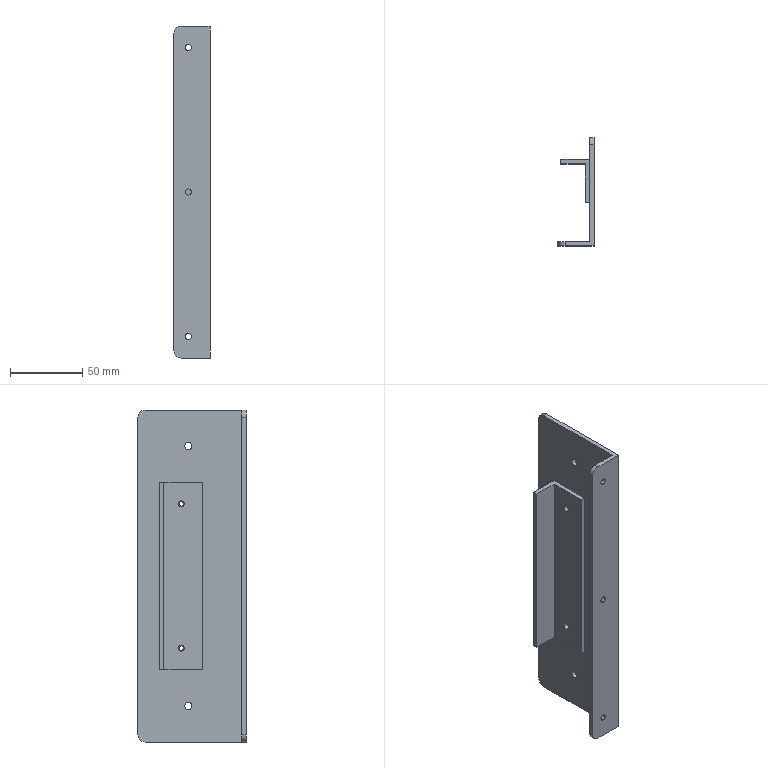Part | SolidWorks | features HoleWzd 4, Fillet 2, FlattenBends 2, ProcessBends 2, BossThin 1, ExtruThin 1 | 2 solids | 38 faces | box 25 x 75 x 230 mm | volume 84822 mm3 | cylinder 22 | plane 16 | commonest cylinder face diameters 4.2 x10 3.2 x4 5 x4 10 x4
STEP:
#1=CARTESIAN_POINT('',(22.,45.,-47.9));
#2=VERTEX_POINT('',#1);
#3=CARTESIAN_POINT('',(22.,45.,-52.1));
#4=VERTEX_POINT('',#3);
#5=CARTESIAN_POINT('',(22.,45.,-50.));
#6=DIRECTION('',(1.,0.,0.));
#7=DIRECTION('',(0.,1.,0.));
#8=AXIS2_PLACEMENT_3D('',#5,#6,#7);
#9=CIRCLE('',#8,2.1);
#10=EDGE_CURVE('',#2,#4,#9,.T.);
#11=ORIENTED_EDGE('',*,*,#10,.T.);
#12=CARTESIAN_POINT('',(19.,45.,-52.1));
#13=VERTEX_POINT('',#12);
#14=CARTESIAN_POINT('',(19.,45.,-52.1));
#15=DIRECTION('',(-1.,0.,0.));
#16=VECTOR('',#15,1000.);
#17=LINE('',#14,#16);
#18=EDGE_CURVE('',#4,#13,#17,.T.);
#19=ORIENTED_EDGE('',*,*,#18,.T.);
#20=CARTESIAN_POINT('',(19.,45.,-47.9));
#21=VERTEX_POINT('',#20);
#22=CARTESIAN_POINT('',(19.,45.,-50.));
#23=DIRECTION('',(-1.,0.,0.));
#24=DIRECTION('',(0.,0.,1.));
#25=AXIS2_PLACEMENT_3D('',#22,#23,#24);
#26=CIRCLE('',#25,2.1);
#27=EDGE_CURVE('',#13,#21,#26,.T.);
#28=ORIENTED_EDGE('',*,*,#27,.T.);
#29=CARTESIAN_POINT('',(19.,45.,-47.9));
#30=DIRECTION('',(-1.,0.,0.));
#31=VECTOR('',#30,1000.);
#32=LINE('',#29,#31);
#33=EDGE_CURVE('',#2,#21,#32,.T.);
#34=ORIENTED_EDGE('',*,*,#33,.F.);
#35=EDGE_LOOP('',(#11,#19,#28,#34));
#36=FACE_OUTER_BOUND('',#35,.T.);
#37=CARTESIAN_POINT('',(19.,45.,-50.));
#38=DIRECTION('',(-1.,0.,0.));
#39=DIRECTION('',(0.,0.,1.));
#40=AXIS2_PLACEMENT_3D('',#37,#38,#39);
#41=CYLINDRICAL_SURFACE('',#40,2.1);
#42=ADVANCED_FACE('',(#36),#41,.F.);
#43=CARTESIAN_POINT('',(22.,45.,52.1));
#44=VERTEX_POINT('',#43);
#45=CARTESIAN_POINT('',(22.,45.,47.9));
#46=VERTEX_POINT('',#45);
#47=CARTESIAN_POINT('',(22.,45.,50.));
#48=DIRECTION('',(1.,0.,0.));
#49=DIRECTION('',(0.,1.,0.));
#50=AXIS2_PLACEMENT_3D('',#47,#48,#49);
#51=CIRCLE('',#50,2.1);
#52=EDGE_CURVE('',#44,#46,#51,.T.);
#53=ORIENTED_EDGE('',*,*,#52,.T.);
#54=CARTESIAN_POINT('',(19.,45.,47.9));
#55=VERTEX_POINT('',#54);
#56=CARTESIAN_POINT('',(19.,45.,47.9));
#57=DIRECTION('',(-1.,0.,0.));
#58=VECTOR('',#57,1000.);
#59=LINE('',#56,#58);
#60=EDGE_CURVE('',#46,#55,#59,.T.);
#61=ORIENTED_EDGE('',*,*,#60,.T.);
#62=CARTESIAN_POINT('',(19.,45.,52.1));
#63=VERTEX_POINT('',#62);
#64=CARTESIAN_POINT('',(19.,45.,50.));
#65=DIRECTION('',(-1.,0.,0.));
#66=DIRECTION('',(0.,0.,1.));
#67=AXIS2_PLACEMENT_3D('',#64,#65,#66);
#68=CIRCLE('',#67,2.1);
#69=EDGE_CURVE('',#55,#63,#68,.T.);
#70=ORIENTED_EDGE('',*,*,#69,.T.);
#71=CARTESIAN_POINT('',(19.,45.,52.1));
#72=DIRECTION('',(-1.,0.,0.));
#73=VECTOR('',#72,1000.);
#74=LINE('',#71,#73);
#75=EDGE_CURVE('',#44,#63,#74,.T.);
#76=ORIENTED_EDGE('',*,*,#75,.F.);
#77=EDGE_LOOP('',(#53,#61,#70,#76));
#78=FACE_OUTER_BOUND('',#77,.T.);
#79=CARTESIAN_POINT('',(19.,45.,50.));
#80=DIRECTION('',(-1.,0.,0.));
#81=DIRECTION('',(0.,0.,1.));
#82=AXIS2_PLACEMENT_3D('',#79,#80,#81);
#83=CYLINDRICAL_SURFACE('',#82,2.1);
#84=ADVANCED_FACE('',(#78),#83,.F.);
#85=CARTESIAN_POINT('',(19.,45.,-50.));
#86=DIRECTION('',(-1.,0.,0.));
#87=DIRECTION('',(0.,0.,1.));
#88=AXIS2_PLACEMENT_3D('',#85,#86,#87);
#89=CIRCLE('',#88,2.1);
#90=EDGE_CURVE('',#21,#13,#89,.T.);
#91=ORIENTED_EDGE('',*,*,#90,.F.);
#92=ORIENTED_EDGE('',*,*,#27,.F.);
#93=EDGE_LOOP('',(#91,#92));
#94=FACE_BOUND('',#93,.T.);
#95=CARTESIAN_POINT('',(19.,45.,50.));
#96=DIRECTION('',(-1.,0.,0.));
#97=DIRECTION('',(0.,0.,1.));
#98=AXIS2_PLACEMENT_3D('',#95,#96,#97);
#99=CIRCLE('',#98,2.1);
#100=EDGE_CURVE('',#63,#55,#99,.T.);
#101=ORIENTED_EDGE('',*,*,#100,.F.);
#102=ORIENTED_EDGE('',*,*,#69,.F.);
#103=EDGE_LOOP('',(#101,#102));
#104=FACE_BOUND('',#103,.T.);
#105=CARTESIAN_POINT('',(19.,57.,-65.));
#106=VERTEX_POINT('',#105);
#107=CARTESIAN_POINT('',(19.,30.,-65.));
#108=VERTEX_POINT('',#107);
#109=CARTESIAN_POINT('',(19.,60.,-65.));
#110=DIRECTION('',(0.,-1.,0.));
#111=VECTOR('',#110,1000.);
#112=LINE('',#109,#111);
#113=EDGE_CURVE('',#106,#108,#112,.T.);
#114=ORIENTED_EDGE('',*,*,#113,.T.);
#115=CARTESIAN_POINT('',(19.,30.,65.));
#116=VERTEX_POINT('',#115);
#117=CARTESIAN_POINT('',(19.,30.,65.));
#118=DIRECTION('',(0.,0.,-1.));
#119=VECTOR('',#118,1000.);
#120=LINE('',#117,#119);
#121=EDGE_CURVE('',#116,#108,#120,.T.);
#122=ORIENTED_EDGE('',*,*,#121,.F.);
#123=CARTESIAN_POINT('',(19.,57.,65.));
#124=VERTEX_POINT('',#123);
#125=CARTESIAN_POINT('',(19.,60.,65.));
#126=DIRECTION('',(0.,-1.,0.));
#127=VECTOR('',#126,1000.);
#128=LINE('',#125,#127);
#129=EDGE_CURVE('',#124,#116,#128,.T.);
#130=ORIENTED_EDGE('',*,*,#129,.F.);
#131=CARTESIAN_POINT('',(19.,57.,65.));
#132=DIRECTION('',(0.,0.,-1.));
#133=VECTOR('',#132,1000.);
#134=LINE('',#131,#133);
#135=EDGE_CURVE('',#124,#106,#134,.T.);
#136=ORIENTED_EDGE('',*,*,#135,.T.);
#137=EDGE_LOOP('',(#114,#122,#130,#136));
#138=FACE_OUTER_BOUND('',#137,.T.);
#139=CARTESIAN_POINT('',(19.,60.,65.));
#140=DIRECTION('',(1.,0.,0.));
#141=DIRECTION('',(0.,1.,0.));
#142=AXIS2_PLACEMENT_3D('',#139,#140,#141);
#143=PLANE('',#142);
#144=ADVANCED_FACE('',(#94,#104,#138),#143,.F.);
#145=CARTESIAN_POINT('',(22.,30.,-65.));
#146=VERTEX_POINT('',#145);
#147=CARTESIAN_POINT('',(22.,30.,-65.));
#148=DIRECTION('',(-1.,0.,0.));
#149=VECTOR('',#148,1000.);
#150=LINE('',#147,#149);
#151=EDGE_CURVE('',#146,#108,#150,.T.);
#152=ORIENTED_EDGE('',*,*,#151,.F.);
#153=CARTESIAN_POINT('',(22.,30.,65.));
#154=VERTEX_POINT('',#153);
#155=CARTESIAN_POINT('',(22.,30.,65.));
#156=DIRECTION('',(0.,0.,-1.));
#157=VECTOR('',#156,1000.);
#158=LINE('',#155,#157);
#159=EDGE_CURVE('',#154,#146,#158,.T.);
#160=ORIENTED_EDGE('',*,*,#159,.F.);
#161=CARTESIAN_POINT('',(22.,30.,65.));
#162=DIRECTION('',(-1.,0.,0.));
#163=VECTOR('',#162,1000.);
#164=LINE('',#161,#163);
#165=EDGE_CURVE('',#154,#116,#164,.T.);
#166=ORIENTED_EDGE('',*,*,#165,.T.);
#167=ORIENTED_EDGE('',*,*,#121,.T.);
#168=EDGE_LOOP('',(#152,#160,#166,#167));
#169=FACE_OUTER_BOUND('',#168,.T.);
#170=CARTESIAN_POINT('',(22.,30.,65.));
#171=DIRECTION('',(0.,-1.,0.));
#172=DIRECTION('',(0.,0.,-1.));
#173=AXIS2_PLACEMENT_3D('',#170,#171,#172);
#174=PLANE('',#173);
#175=ADVANCED_FACE('',(#169),#174,.T.);
#176=ORIENTED_EDGE('',*,*,#10,.F.);
#177=CARTESIAN_POINT('',(22.,45.,-50.));
#178=DIRECTION('',(1.,0.,0.));
#179=DIRECTION('',(0.,1.,0.));
#180=AXIS2_PLACEMENT_3D('',#177,#178,#179);
#181=CIRCLE('',#180,2.1);
#182=EDGE_CURVE('',#4,#2,#181,.T.);
#183=ORIENTED_EDGE('',*,*,#182,.F.);
#184=EDGE_LOOP('',(#176,#183));
#185=FACE_BOUND('',#184,.T.);
#186=ORIENTED_EDGE('',*,*,#52,.F.);
#187=CARTESIAN_POINT('',(22.,45.,50.));
#188=DIRECTION('',(1.,0.,0.));
#189=DIRECTION('',(0.,1.,0.));
#190=AXIS2_PLACEMENT_3D('',#187,#188,#189);
#191=CIRCLE('',#190,2.1);
#192=EDGE_CURVE('',#46,#44,#191,.T.);
#193=ORIENTED_EDGE('',*,*,#192,.F.);
#194=EDGE_LOOP('',(#186,#193));
#195=FACE_BOUND('',#194,.T.);
#196=CARTESIAN_POINT('',(22.,60.,-65.));
#197=VERTEX_POINT('',#196);
#198=CARTESIAN_POINT('',(22.,60.,-65.));
#199=DIRECTION('',(0.,-1.,0.));
#200=VECTOR('',#199,1000.);
#201=LINE('',#198,#200);
#202=EDGE_CURVE('',#197,#146,#201,.T.);
#203=ORIENTED_EDGE('',*,*,#202,.F.);
#204=CARTESIAN_POINT('',(22.,60.,65.));
#205=VERTEX_POINT('',#204);
#206=CARTESIAN_POINT('',(22.,60.,65.));
#207=DIRECTION('',(0.,0.,-1.));
#208=VECTOR('',#207,1000.);
#209=LINE('',#206,#208);
#210=EDGE_CURVE('',#205,#197,#209,.T.);
#211=ORIENTED_EDGE('',*,*,#210,.F.);
#212=CARTESIAN_POINT('',(22.,60.,65.));
#213=DIRECTION('',(0.,-1.,0.));
#214=VECTOR('',#213,1000.);
#215=LINE('',#212,#214);
#216=EDGE_CURVE('',#205,#154,#215,.T.);
#217=ORIENTED_EDGE('',*,*,#216,.T.);
#218=ORIENTED_EDGE('',*,*,#159,.T.);
#219=EDGE_LOOP('',(#203,#211,#217,#218));
#220=FACE_OUTER_BOUND('',#219,.T.);
#221=CARTESIAN_POINT('',(22.,60.,65.));
#222=DIRECTION('',(1.,0.,0.));
#223=DIRECTION('',(0.,1.,0.));
#224=AXIS2_PLACEMENT_3D('',#221,#222,#223);
#225=PLANE('',#224);
#226=ADVANCED_FACE('',(#185,#195,#220),#225,.T.);
#227=CARTESIAN_POINT('',(2.,60.,-65.));
#228=VERTEX_POINT('',#227);
#229=CARTESIAN_POINT('',(2.,60.,-65.));
#230=DIRECTION('',(1.,0.,0.));
#231=VECTOR('',#230,1000.);
#232=LINE('',#229,#231);
#233=EDGE_CURVE('',#228,#197,#232,.T.);
#234=ORIENTED_EDGE('',*,*,#233,.F.);
#235=CARTESIAN_POINT('',(2.,60.,65.));
#236=VERTEX_POINT('',#235);
#237=CARTESIAN_POINT('',(2.,60.,65.));
#238=DIRECTION('',(0.,0.,-1.));
#239=VECTOR('',#238,1000.);
#240=LINE('',#237,#239);
#241=EDGE_CURVE('',#236,#228,#240,.T.);
#242=ORIENTED_EDGE('',*,*,#241,.F.);
#243=CARTESIAN_POINT('',(2.,60.,65.));
#244=DIRECTION('',(1.,0.,0.));
#245=VECTOR('',#244,1000.);
#246=LINE('',#243,#245);
#247=EDGE_CURVE('',#236,#205,#246,.T.);
#248=ORIENTED_EDGE('',*,*,#247,.T.);
#249=ORIENTED_EDGE('',*,*,#210,.T.);
#250=EDGE_LOOP('',(#234,#242,#248,#249));
#251=FACE_OUTER_BOUND('',#250,.T.);
#252=CARTESIAN_POINT('',(2.,60.,65.));
#253=DIRECTION('',(0.,1.,0.));
#254=DIRECTION('',(0.,0.,1.));
#255=AXIS2_PLACEMENT_3D('',#252,#253,#254);
#256=PLANE('',#255);
#257=ADVANCED_FACE('',(#251),#256,.T.);
#258=CARTESIAN_POINT('',(2.,57.,-65.));
#259=VERTEX_POINT('',#258);
#260=CARTESIAN_POINT('',(2.,57.,-65.));
#261=DIRECTION('',(0.,1.,0.));
#262=VECTOR('',#261,1000.);
#263=LINE('',#260,#262);
#264=EDGE_CURVE('',#259,#228,#263,.T.);
#265=ORIENTED_EDGE('',*,*,#264,.F.);
#266=CARTESIAN_POINT('',(2.,57.,65.));
#267=VERTEX_POINT('',#266);
#268=CARTESIAN_POINT('',(2.,57.,65.));
#269=DIRECTION('',(0.,0.,-1.));
#270=VECTOR('',#269,1000.);
#271=LINE('',#268,#270);
#272=EDGE_CURVE('',#267,#259,#271,.T.);
#273=ORIENTED_EDGE('',*,*,#272,.F.);
#274=CARTESIAN_POINT('',(2.,57.,65.));
#275=DIRECTION('',(0.,1.,0.));
#276=VECTOR('',#275,1000.);
#277=LINE('',#274,#276);
#278=EDGE_CURVE('',#267,#236,#277,.T.);
#279=ORIENTED_EDGE('',*,*,#278,.T.);
#280=ORIENTED_EDGE('',*,*,#241,.T.);
#281=EDGE_LOOP('',(#265,#273,#279,#280));
#282=FACE_OUTER_BOUND('',#281,.T.);
#283=CARTESIAN_POINT('',(2.,57.,65.));
#284=DIRECTION('',(-1.,0.,0.));
#285=DIRECTION('',(0.,0.,1.));
#286=AXIS2_PLACEMENT_3D('',#283,#284,#285);
#287=PLANE('',#286);
#288=ADVANCED_FACE('',(#282),#287,.T.);
#289=CARTESIAN_POINT('',(2.,57.,-65.));
#290=DIRECTION('',(1.,0.,0.));
#291=VECTOR('',#290,1000.);
#292=LINE('',#289,#291);
#293=EDGE_CURVE('',#259,#106,#292,.T.);
#294=ORIENTED_EDGE('',*,*,#293,.T.);
#295=ORIENTED_EDGE('',*,*,#135,.F.);
#296=CARTESIAN_POINT('',(2.,57.,65.));
#297=DIRECTION('',(1.,0.,0.));
#298=VECTOR('',#297,1000.);
#299=LINE('',#296,#298);
#300=EDGE_CURVE('',#267,#124,#299,.T.);
#301=ORIENTED_EDGE('',*,*,#300,.F.);
#302=ORIENTED_EDGE('',*,*,#272,.T.);
#303=EDGE_LOOP('',(#294,#295,#301,#302));
#304=FACE_OUTER_BOUND('',#303,.T.);
#305=CARTESIAN_POINT('',(2.,57.,65.));
#306=DIRECTION('',(0.,1.,0.));
#307=DIRECTION('',(0.,0.,1.));
#308=AXIS2_PLACEMENT_3D('',#305,#306,#307);
#309=PLANE('',#308);
#310=ADVANCED_FACE('',(#304),#309,.F.);
#311=ORIENTED_EDGE('',*,*,#129,.T.);
#312=ORIENTED_EDGE('',*,*,#165,.F.);
#313=ORIENTED_EDGE('',*,*,#216,.F.);
#314=ORIENTED_EDGE('',*,*,#247,.F.);
#315=ORIENTED_EDGE('',*,*,#278,.F.);
#316=ORIENTED_EDGE('',*,*,#300,.T.);
#317=EDGE_LOOP('',(#311,#312,#313,#314,#315,#316));
#318=FACE_OUTER_BOUND('',#317,.T.);
#319=CARTESIAN_POINT('',(0.,0.,65.));
#320=DIRECTION('',(0.,0.,-1.));
#321=DIRECTION('',(-1.,0.,0.));
#322=AXIS2_PLACEMENT_3D('',#319,#320,#321);
#323=PLANE('',#322);
#324=ADVANCED_FACE('',(#318),#323,.F.);
#325=ORIENTED_EDGE('',*,*,#113,.F.);
#326=ORIENTED_EDGE('',*,*,#293,.F.);
#327=ORIENTED_EDGE('',*,*,#264,.T.);
#328=ORIENTED_EDGE('',*,*,#233,.T.);
#329=ORIENTED_EDGE('',*,*,#202,.T.);
#330=ORIENTED_EDGE('',*,*,#151,.T.);
#331=EDGE_LOOP('',(#325,#326,#327,#328,#329,#330));
#332=FACE_OUTER_BOUND('',#331,.T.);
#333=CARTESIAN_POINT('',(0.,0.,-65.));
#334=DIRECTION('',(0.,0.,-1.));
#335=DIRECTION('',(-1.,0.,0.));
#336=AXIS2_PLACEMENT_3D('',#333,#334,#335);
#337=PLANE('',#336);
#338=ADVANCED_FACE('',(#332),#337,.T.);
#339=ORIENTED_EDGE('',*,*,#60,.F.);
#340=ORIENTED_EDGE('',*,*,#192,.T.);
#341=ORIENTED_EDGE('',*,*,#75,.T.);
#342=ORIENTED_EDGE('',*,*,#100,.T.);
#343=EDGE_LOOP('',(#339,#340,#341,#342));
#344=FACE_OUTER_BOUND('',#343,.T.);
#345=CARTESIAN_POINT('',(19.,45.,50.));
#346=DIRECTION('',(-1.,0.,0.));
#347=DIRECTION('',(0.,0.,1.));
#348=AXIS2_PLACEMENT_3D('',#345,#346,#347);
#349=CYLINDRICAL_SURFACE('',#348,2.1);
#350=ADVANCED_FACE('',(#344),#349,.F.);
#351=ORIENTED_EDGE('',*,*,#18,.F.);
#352=ORIENTED_EDGE('',*,*,#182,.T.);
#353=ORIENTED_EDGE('',*,*,#33,.T.);
#354=ORIENTED_EDGE('',*,*,#90,.T.);
#355=EDGE_LOOP('',(#351,#352,#353,#354));
#356=FACE_OUTER_BOUND('',#355,.T.);
#357=CARTESIAN_POINT('',(19.,45.,-50.));
#358=DIRECTION('',(-1.,0.,0.));
#359=DIRECTION('',(0.,0.,1.));
#360=AXIS2_PLACEMENT_3D('',#357,#358,#359);
#361=CYLINDRICAL_SURFACE('',#360,2.1);
#362=ADVANCED_FACE('',(#356),#361,.F.);
#363=CLOSED_SHELL('',(#42,#84,#144,#175,#226,#257,#288,#310,#324,#338,#350,#362));
#364=MANIFOLD_SOLID_BREP('',#363);
#365=CARTESIAN_POINT('',(25.,45.,-51.6));
#366=VERTEX_POINT('',#365);
#367=CARTESIAN_POINT('',(25.,45.,-48.4));
#368=VERTEX_POINT('',#367);
#369=CARTESIAN_POINT('',(25.,45.,-50.));
#370=DIRECTION('',(-1.,0.,0.));
#371=DIRECTION('',(0.,0.,1.));
#372=AXIS2_PLACEMENT_3D('',#369,#370,#371);
#373=CIRCLE('',#372,1.6);
#374=EDGE_CURVE('',#366,#368,#373,.T.);
#375=ORIENTED_EDGE('',*,*,#374,.F.);
#376=CARTESIAN_POINT('',(22.,45.,-51.6));
#377=VERTEX_POINT('',#376);
#378=CARTESIAN_POINT('',(22.,45.,-51.6));
#379=DIRECTION('',(-1.,0.,0.));
#380=VECTOR('',#379,1000.);
#381=LINE('',#378,#380);
#382=EDGE_CURVE('',#366,#377,#381,.T.);
#383=ORIENTED_EDGE('',*,*,#382,.T.);
#384=CARTESIAN_POINT('',(22.,45.,-48.4));
#385=VERTEX_POINT('',#384);
#386=CARTESIAN_POINT('',(22.,45.,-50.));
#387=DIRECTION('',(-1.,0.,0.));
#388=DIRECTION('',(0.,0.,1.));
#389=AXIS2_PLACEMENT_3D('',#386,#387,#388);
#390=CIRCLE('',#389,1.6);
#391=EDGE_CURVE('',#377,#385,#390,.T.);
#392=ORIENTED_EDGE('',*,*,#391,.T.);
#393=CARTESIAN_POINT('',(22.,45.,-48.4));
#394=DIRECTION('',(-1.,0.,0.));
#395=VECTOR('',#394,1000.);
#396=LINE('',#393,#395);
#397=EDGE_CURVE('',#368,#385,#396,.T.);
#398=ORIENTED_EDGE('',*,*,#397,.F.);
#399=EDGE_LOOP('',(#375,#383,#392,#398));
#400=FACE_OUTER_BOUND('',#399,.T.);
#401=CARTESIAN_POINT('',(22.,45.,-50.));
#402=DIRECTION('',(-1.,0.,0.));
#403=DIRECTION('',(0.,0.,1.));
#404=AXIS2_PLACEMENT_3D('',#401,#402,#403);
#405=CYLINDRICAL_SURFACE('',#404,1.6);
#406=ADVANCED_FACE('',(#400),#405,.F.);
#407=CARTESIAN_POINT('',(25.,45.,48.4));
#408=VERTEX_POINT('',#407);
#409=CARTESIAN_POINT('',(25.,45.,51.6));
#410=VERTEX_POINT('',#409);
#411=CARTESIAN_POINT('',(25.,45.,50.));
#412=DIRECTION('',(-1.,0.,0.));
#413=DIRECTION('',(0.,0.,1.));
#414=AXIS2_PLACEMENT_3D('',#411,#412,#413);
#415=CIRCLE('',#414,1.6);
#416=EDGE_CURVE('',#408,#410,#415,.T.);
#417=ORIENTED_EDGE('',*,*,#416,.F.);
#418=CARTESIAN_POINT('',(22.,45.,48.4));
#419=VERTEX_POINT('',#418);
#420=CARTESIAN_POINT('',(22.,45.,48.4));
#421=DIRECTION('',(-1.,0.,0.));
#422=VECTOR('',#421,1000.);
#423=LINE('',#420,#422);
#424=EDGE_CURVE('',#408,#419,#423,.T.);
#425=ORIENTED_EDGE('',*,*,#424,.T.);
#426=CARTESIAN_POINT('',(22.,45.,51.6));
#427=VERTEX_POINT('',#426);
#428=CARTESIAN_POINT('',(22.,45.,50.));
#429=DIRECTION('',(-1.,0.,0.));
#430=DIRECTION('',(0.,0.,1.));
#431=AXIS2_PLACEMENT_3D('',#428,#429,#430);
#432=CIRCLE('',#431,1.6);
#433=EDGE_CURVE('',#419,#427,#432,.T.);
#434=ORIENTED_EDGE('',*,*,#433,.T.);
#435=CARTESIAN_POINT('',(22.,45.,51.6));
#436=DIRECTION('',(-1.,0.,0.));
#437=VECTOR('',#436,1000.);
#438=LINE('',#435,#437);
#439=EDGE_CURVE('',#410,#427,#438,.T.);
#440=ORIENTED_EDGE('',*,*,#439,.F.);
#441=EDGE_LOOP('',(#417,#425,#434,#440));
#442=FACE_OUTER_BOUND('',#441,.T.);
#443=CARTESIAN_POINT('',(22.,45.,50.));
#444=DIRECTION('',(-1.,0.,0.));
#445=DIRECTION('',(0.,0.,1.));
#446=AXIS2_PLACEMENT_3D('',#443,#444,#445);
#447=CYLINDRICAL_SURFACE('',#446,1.6);
#448=ADVANCED_FACE('',(#442),#447,.F.);
#449=CARTESIAN_POINT('',(25.,40.,-92.5));
#450=VERTEX_POINT('',#449);
#451=CARTESIAN_POINT('',(25.,40.,-87.5));
#452=VERTEX_POINT('',#451);
#453=CARTESIAN_POINT('',(25.,40.,-90.));
#454=DIRECTION('',(-1.,0.,0.));
#455=DIRECTION('',(0.,0.,1.));
#456=AXIS2_PLACEMENT_3D('',#453,#454,#455);
#457=CIRCLE('',#456,2.5);
#458=EDGE_CURVE('',#450,#452,#457,.T.);
#459=ORIENTED_EDGE('',*,*,#458,.F.);
#460=CARTESIAN_POINT('',(22.,40.,-92.5));
#461=VERTEX_POINT('',#460);
#462=CARTESIAN_POINT('',(22.,40.,-92.5));
#463=DIRECTION('',(-1.,0.,0.));
#464=VECTOR('',#463,1000.);
#465=LINE('',#462,#464);
#466=EDGE_CURVE('',#450,#461,#465,.T.);
#467=ORIENTED_EDGE('',*,*,#466,.T.);
#468=CARTESIAN_POINT('',(22.,40.,-87.5));
#469=VERTEX_POINT('',#468);
#470=CARTESIAN_POINT('',(22.,40.,-90.));
#471=DIRECTION('',(-1.,0.,0.));
#472=DIRECTION('',(0.,0.,1.));
#473=AXIS2_PLACEMENT_3D('',#470,#471,#472);
#474=CIRCLE('',#473,2.5);
#475=EDGE_CURVE('',#461,#469,#474,.T.);
#476=ORIENTED_EDGE('',*,*,#475,.T.);
#477=CARTESIAN_POINT('',(22.,40.,-87.5));
#478=DIRECTION('',(-1.,0.,0.));
#479=VECTOR('',#478,1000.);
#480=LINE('',#477,#479);
#481=EDGE_CURVE('',#452,#469,#480,.T.);
#482=ORIENTED_EDGE('',*,*,#481,.F.);
#483=EDGE_LOOP('',(#459,#467,#476,#482));
#484=FACE_OUTER_BOUND('',#483,.T.);
#485=CARTESIAN_POINT('',(22.,40.,-90.));
#486=DIRECTION('',(-1.,0.,0.));
#487=DIRECTION('',(0.,0.,1.));
#488=AXIS2_PLACEMENT_3D('',#485,#486,#487);
#489=CYLINDRICAL_SURFACE('',#488,2.5);
#490=ADVANCED_FACE('',(#484),#489,.F.);
#491=CARTESIAN_POINT('',(25.,40.,87.5));
#492=VERTEX_POINT('',#491);
#493=CARTESIAN_POINT('',(25.,40.,92.5));
#494=VERTEX_POINT('',#493);
#495=CARTESIAN_POINT('',(25.,40.,90.));
#496=DIRECTION('',(-1.,0.,0.));
#497=DIRECTION('',(0.,0.,1.));
#498=AXIS2_PLACEMENT_3D('',#495,#496,#497);
#499=CIRCLE('',#498,2.5);
#500=EDGE_CURVE('',#492,#494,#499,.T.);
#501=ORIENTED_EDGE('',*,*,#500,.F.);
#502=CARTESIAN_POINT('',(22.,40.,87.5));
#503=VERTEX_POINT('',#502);
#504=CARTESIAN_POINT('',(22.,40.,87.5));
#505=DIRECTION('',(-1.,0.,0.));
#506=VECTOR('',#505,1000.);
#507=LINE('',#504,#506);
#508=EDGE_CURVE('',#492,#503,#507,.T.);
#509=ORIENTED_EDGE('',*,*,#508,.T.);
#510=CARTESIAN_POINT('',(22.,40.,92.5));
#511=VERTEX_POINT('',#510);
#512=CARTESIAN_POINT('',(22.,40.,90.));
#513=DIRECTION('',(-1.,0.,0.));
#514=DIRECTION('',(0.,0.,1.));
#515=AXIS2_PLACEMENT_3D('',#512,#513,#514);
#516=CIRCLE('',#515,2.5);
#517=EDGE_CURVE('',#503,#511,#516,.T.);
#518=ORIENTED_EDGE('',*,*,#517,.T.);
#519=CARTESIAN_POINT('',(22.,40.,92.5));
#520=DIRECTION('',(-1.,0.,0.));
#521=VECTOR('',#520,1000.);
#522=LINE('',#519,#521);
#523=EDGE_CURVE('',#494,#511,#522,.T.);
#524=ORIENTED_EDGE('',*,*,#523,.F.);
#525=EDGE_LOOP('',(#501,#509,#518,#524));
#526=FACE_OUTER_BOUND('',#525,.T.);
#527=CARTESIAN_POINT('',(22.,40.,90.));
#528=DIRECTION('',(-1.,0.,0.));
#529=DIRECTION('',(0.,0.,1.));
#530=AXIS2_PLACEMENT_3D('',#527,#528,#529);
#531=CYLINDRICAL_SURFACE('',#530,2.5);
#532=ADVANCED_FACE('',(#526),#531,.F.);
#533=CARTESIAN_POINT('',(10.,0.,-102.1));
#534=VERTEX_POINT('',#533);
#535=CARTESIAN_POINT('',(10.,0.,-97.9));
#536=VERTEX_POINT('',#535);
#537=CARTESIAN_POINT('',(10.,0.,-100.));
#538=DIRECTION('',(0.,1.,0.));
#539=DIRECTION('',(0.,0.,1.));
#540=AXIS2_PLACEMENT_3D('',#537,#538,#539);
#541=CIRCLE('',#540,2.1);
#542=EDGE_CURVE('',#534,#536,#541,.T.);
#543=ORIENTED_EDGE('',*,*,#542,.F.);
#544=CARTESIAN_POINT('',(10.,3.,-102.1));
#545=VERTEX_POINT('',#544);
#546=CARTESIAN_POINT('',(10.,3.,-102.1));
#547=DIRECTION('',(0.,1.,0.));
#548=VECTOR('',#547,1000.);
#549=LINE('',#546,#548);
#550=EDGE_CURVE('',#534,#545,#549,.T.);
#551=ORIENTED_EDGE('',*,*,#550,.T.);
#552=CARTESIAN_POINT('',(10.,3.,-97.9));
#553=VERTEX_POINT('',#552);
#554=CARTESIAN_POINT('',(10.,3.,-100.));
#555=DIRECTION('',(0.,1.,0.));
#556=DIRECTION('',(0.,0.,1.));
#557=AXIS2_PLACEMENT_3D('',#554,#555,#556);
#558=CIRCLE('',#557,2.1);
#559=EDGE_CURVE('',#545,#553,#558,.T.);
#560=ORIENTED_EDGE('',*,*,#559,.T.);
#561=CARTESIAN_POINT('',(10.,3.,-97.9));
#562=DIRECTION('',(0.,1.,0.));
#563=VECTOR('',#562,1000.);
#564=LINE('',#561,#563);
#565=EDGE_CURVE('',#536,#553,#564,.T.);
#566=ORIENTED_EDGE('',*,*,#565,.F.);
#567=EDGE_LOOP('',(#543,#551,#560,#566));
#568=FACE_OUTER_BOUND('',#567,.T.);
#569=CARTESIAN_POINT('',(10.,3.,-100.));
#570=DIRECTION('',(0.,1.,0.));
#571=DIRECTION('',(0.,0.,1.));
#572=AXIS2_PLACEMENT_3D('',#569,#570,#571);
#573=CYLINDRICAL_SURFACE('',#572,2.1);
#574=ADVANCED_FACE('',(#568),#573,.F.);
#575=CARTESIAN_POINT('',(10.,0.,97.9));
#576=VERTEX_POINT('',#575);
#577=CARTESIAN_POINT('',(10.,0.,102.1));
#578=VERTEX_POINT('',#577);
#579=CARTESIAN_POINT('',(10.,0.,100.));
#580=DIRECTION('',(0.,1.,0.));
#581=DIRECTION('',(0.,0.,1.));
#582=AXIS2_PLACEMENT_3D('',#579,#580,#581);
#583=CIRCLE('',#582,2.1);
#584=EDGE_CURVE('',#576,#578,#583,.T.);
#585=ORIENTED_EDGE('',*,*,#584,.F.);
#586=CARTESIAN_POINT('',(10.,3.,97.9));
#587=VERTEX_POINT('',#586);
#588=CARTESIAN_POINT('',(10.,3.,97.9));
#589=DIRECTION('',(0.,1.,0.));
#590=VECTOR('',#589,1000.);
#591=LINE('',#588,#590);
#592=EDGE_CURVE('',#576,#587,#591,.T.);
#593=ORIENTED_EDGE('',*,*,#592,.T.);
#594=CARTESIAN_POINT('',(10.,3.,102.1));
#595=VERTEX_POINT('',#594);
#596=CARTESIAN_POINT('',(10.,3.,100.));
#597=DIRECTION('',(0.,1.,0.));
#598=DIRECTION('',(0.,0.,1.));
#599=AXIS2_PLACEMENT_3D('',#596,#597,#598);
#600=CIRCLE('',#599,2.1);
#601=EDGE_CURVE('',#587,#595,#600,.T.);
#602=ORIENTED_EDGE('',*,*,#601,.T.);
#603=CARTESIAN_POINT('',(10.,3.,102.1));
#604=DIRECTION('',(0.,1.,0.));
#605=VECTOR('',#604,1000.);
#606=LINE('',#603,#605);
#607=EDGE_CURVE('',#578,#595,#606,.T.);
#608=ORIENTED_EDGE('',*,*,#607,.F.);
#609=EDGE_LOOP('',(#585,#593,#602,#608));
#610=FACE_OUTER_BOUND('',#609,.T.);
#611=CARTESIAN_POINT('',(10.,3.,100.));
#612=DIRECTION('',(0.,1.,0.));
#613=DIRECTION('',(0.,0.,1.));
#614=AXIS2_PLACEMENT_3D('',#611,#612,#613);
#615=CYLINDRICAL_SURFACE('',#614,2.1);
#616=ADVANCED_FACE('',(#610),#615,.F.);
#617=CARTESIAN_POINT('',(10.,0.,-2.1));
#618=VERTEX_POINT('',#617);
#619=CARTESIAN_POINT('',(10.,0.,2.1));
#620=VERTEX_POINT('',#619);
#621=CARTESIAN_POINT('',(10.,0.,0.));
#622=DIRECTION('',(0.,1.,0.));
#623=DIRECTION('',(0.,0.,1.));
#624=AXIS2_PLACEMENT_3D('',#621,#622,#623);
#625=CIRCLE('',#624,2.1);
#626=EDGE_CURVE('',#618,#620,#625,.T.);
#627=ORIENTED_EDGE('',*,*,#626,.F.);
#628=CARTESIAN_POINT('',(10.,3.,-2.1));
#629=VERTEX_POINT('',#628);
#630=CARTESIAN_POINT('',(10.,3.,-2.1));
#631=DIRECTION('',(0.,1.,0.));
#632=VECTOR('',#631,1000.);
#633=LINE('',#630,#632);
#634=EDGE_CURVE('',#618,#629,#633,.T.);
#635=ORIENTED_EDGE('',*,*,#634,.T.);
#636=CARTESIAN_POINT('',(10.,3.,2.1));
#637=VERTEX_POINT('',#636);
#638=CARTESIAN_POINT('',(10.,3.,0.));
#639=DIRECTION('',(0.,1.,0.));
#640=DIRECTION('',(0.,0.,1.));
#641=AXIS2_PLACEMENT_3D('',#638,#639,#640);
#642=CIRCLE('',#641,2.1);
#643=EDGE_CURVE('',#629,#637,#642,.T.);
#644=ORIENTED_EDGE('',*,*,#643,.T.);
#645=CARTESIAN_POINT('',(10.,3.,2.1));
#646=DIRECTION('',(0.,1.,0.));
#647=VECTOR('',#646,1000.);
#648=LINE('',#645,#647);
#649=EDGE_CURVE('',#620,#637,#648,.T.);
#650=ORIENTED_EDGE('',*,*,#649,.F.);
#651=EDGE_LOOP('',(#627,#635,#644,#650));
#652=FACE_OUTER_BOUND('',#651,.T.);
#653=CARTESIAN_POINT('',(10.,3.,0.));
#654=DIRECTION('',(0.,1.,0.));
#655=DIRECTION('',(0.,0.,1.));
#656=AXIS2_PLACEMENT_3D('',#653,#654,#655);
#657=CYLINDRICAL_SURFACE('',#656,2.1);
#658=ADVANCED_FACE('',(#652),#657,.F.);
#659=CARTESIAN_POINT('',(25.,45.,-50.));
#660=DIRECTION('',(-1.,0.,0.));
#661=DIRECTION('',(0.,0.,1.));
#662=AXIS2_PLACEMENT_3D('',#659,#660,#661);
#663=CIRCLE('',#662,1.6);
#664=EDGE_CURVE('',#368,#366,#663,.T.);
#665=ORIENTED_EDGE('',*,*,#664,.T.);
#666=ORIENTED_EDGE('',*,*,#374,.T.);
#667=EDGE_LOOP('',(#665,#666));
#668=FACE_BOUND('',#667,.T.);
#669=CARTESIAN_POINT('',(25.,45.,50.));
#670=DIRECTION('',(-1.,0.,0.));
#671=DIRECTION('',(0.,0.,1.));
#672=AXIS2_PLACEMENT_3D('',#669,#670,#671);
#673=CIRCLE('',#672,1.6);
#674=EDGE_CURVE('',#410,#408,#673,.T.);
#675=ORIENTED_EDGE('',*,*,#674,.T.);
#676=ORIENTED_EDGE('',*,*,#416,.T.);
#677=EDGE_LOOP('',(#675,#676));
#678=FACE_BOUND('',#677,.T.);
#679=CARTESIAN_POINT('',(25.,40.,-90.));
#680=DIRECTION('',(-1.,0.,0.));
#681=DIRECTION('',(0.,0.,1.));
#682=AXIS2_PLACEMENT_3D('',#679,#680,#681);
#683=CIRCLE('',#682,2.5);
#684=EDGE_CURVE('',#452,#450,#683,.T.);
#685=ORIENTED_EDGE('',*,*,#684,.T.);
#686=ORIENTED_EDGE('',*,*,#458,.T.);
#687=EDGE_LOOP('',(#685,#686));
#688=FACE_BOUND('',#687,.T.);
#689=CARTESIAN_POINT('',(25.,40.,90.));
#690=DIRECTION('',(-1.,0.,0.));
#691=DIRECTION('',(0.,0.,1.));
#692=AXIS2_PLACEMENT_3D('',#689,#690,#691);
#693=CIRCLE('',#692,2.5);
#694=EDGE_CURVE('',#494,#492,#693,.T.);
#695=ORIENTED_EDGE('',*,*,#694,.T.);
#696=ORIENTED_EDGE('',*,*,#500,.T.);
#697=EDGE_LOOP('',(#695,#696));
#698=FACE_BOUND('',#697,.T.);
#699=CARTESIAN_POINT('',(25.,75.,110.));
#700=VERTEX_POINT('',#699);
#701=CARTESIAN_POINT('',(25.,75.,-110.));
#702=VERTEX_POINT('',#701);
#703=CARTESIAN_POINT('',(25.,75.,115.));
#704=DIRECTION('',(0.,0.,-1.));
#705=VECTOR('',#704,1000.);
#706=LINE('',#703,#705);
#707=EDGE_CURVE('',#700,#702,#706,.T.);
#708=ORIENTED_EDGE('',*,*,#707,.F.);
#709=CARTESIAN_POINT('',(25.,70.,115.));
#710=VERTEX_POINT('',#709);
#711=CARTESIAN_POINT('',(25.,70.,110.));
#712=DIRECTION('',(1.,0.,0.));
#713=DIRECTION('',(0.,0.,1.));
#714=AXIS2_PLACEMENT_3D('',#711,#712,#713);
#715=CIRCLE('',#714,5.);
#716=EDGE_CURVE('',#700,#710,#715,.T.);
#717=ORIENTED_EDGE('',*,*,#716,.T.);
#718=CARTESIAN_POINT('',(25.,0.,115.));
#719=VERTEX_POINT('',#718);
#720=CARTESIAN_POINT('',(25.,0.,115.));
#721=DIRECTION('',(0.,1.,0.));
#722=VECTOR('',#721,1000.);
#723=LINE('',#720,#722);
#724=EDGE_CURVE('',#719,#710,#723,.T.);
#725=ORIENTED_EDGE('',*,*,#724,.F.);
#726=CARTESIAN_POINT('',(25.,0.,-115.));
#727=VERTEX_POINT('',#726);
#728=CARTESIAN_POINT('',(25.,0.,115.));
#729=DIRECTION('',(0.,0.,-1.));
#730=VECTOR('',#729,1000.);
#731=LINE('',#728,#730);
#732=EDGE_CURVE('',#719,#727,#731,.T.);
#733=ORIENTED_EDGE('',*,*,#732,.T.);
#734=CARTESIAN_POINT('',(25.,70.,-115.));
#735=VERTEX_POINT('',#734);
#736=CARTESIAN_POINT('',(25.,0.,-115.));
#737=DIRECTION('',(0.,1.,0.));
#738=VECTOR('',#737,1000.);
#739=LINE('',#736,#738);
#740=EDGE_CURVE('',#727,#735,#739,.T.);
#741=ORIENTED_EDGE('',*,*,#740,.T.);
#742=CARTESIAN_POINT('',(25.,70.,-110.));
#743=DIRECTION('',(1.,0.,0.));
#744=DIRECTION('',(0.,0.,1.));
#745=AXIS2_PLACEMENT_3D('',#742,#743,#744);
#746=CIRCLE('',#745,5.);
#747=EDGE_CURVE('',#735,#702,#746,.T.);
#748=ORIENTED_EDGE('',*,*,#747,.T.);
#749=EDGE_LOOP('',(#708,#717,#725,#733,#741,#748));
#750=FACE_OUTER_BOUND('',#749,.T.);
#751=CARTESIAN_POINT('',(25.,0.,115.));
#752=DIRECTION('',(-1.,0.,0.));
#753=DIRECTION('',(0.,0.,1.));
#754=AXIS2_PLACEMENT_3D('',#751,#752,#753);
#755=PLANE('',#754);
#756=ADVANCED_FACE('',(#668,#678,#688,#698,#750),#755,.F.);
#757=CARTESIAN_POINT('',(22.,75.,110.));
#758=VERTEX_POINT('',#757);
#759=CARTESIAN_POINT('',(22.,75.,-110.));
#760=VERTEX_POINT('',#759);
#761=CARTESIAN_POINT('',(22.,75.,115.));
#762=DIRECTION('',(0.,0.,-1.));
#763=VECTOR('',#762,1000.);
#764=LINE('',#761,#763);
#765=EDGE_CURVE('',#758,#760,#764,.T.);
#766=ORIENTED_EDGE('',*,*,#765,.F.);
#767=CARTESIAN_POINT('',(25.,75.,110.));
#768=DIRECTION('',(1.,0.,0.));
#769=VECTOR('',#768,1000.);
#770=LINE('',#767,#769);
#771=EDGE_CURVE('',#758,#700,#770,.T.);
#772=ORIENTED_EDGE('',*,*,#771,.T.);
#773=ORIENTED_EDGE('',*,*,#707,.T.);
#774=CARTESIAN_POINT('',(22.,75.,-110.));
#775=DIRECTION('',(-1.,0.,0.));
#776=VECTOR('',#775,1000.);
#777=LINE('',#774,#776);
#778=EDGE_CURVE('',#702,#760,#777,.T.);
#779=ORIENTED_EDGE('',*,*,#778,.T.);
#780=EDGE_LOOP('',(#766,#772,#773,#779));
#781=FACE_OUTER_BOUND('',#780,.T.);
#782=CARTESIAN_POINT('',(22.,75.,115.));
#783=DIRECTION('',(0.,1.,0.));
#784=DIRECTION('',(0.,0.,1.));
#785=AXIS2_PLACEMENT_3D('',#782,#783,#784);
#786=PLANE('',#785);
#787=ADVANCED_FACE('',(#781),#786,.T.);
#788=CARTESIAN_POINT('',(22.,45.,-50.));
#789=DIRECTION('',(-1.,0.,0.));
#790=DIRECTION('',(0.,0.,1.));
#791=AXIS2_PLACEMENT_3D('',#788,#789,#790);
#792=CIRCLE('',#791,1.6);
#793=EDGE_CURVE('',#385,#377,#792,.T.);
#794=ORIENTED_EDGE('',*,*,#793,.F.);
#795=ORIENTED_EDGE('',*,*,#391,.F.);
#796=EDGE_LOOP('',(#794,#795));
#797=FACE_BOUND('',#796,.T.);
#798=CARTESIAN_POINT('',(22.,45.,50.));
#799=DIRECTION('',(-1.,0.,0.));
#800=DIRECTION('',(0.,0.,1.));
#801=AXIS2_PLACEMENT_3D('',#798,#799,#800);
#802=CIRCLE('',#801,1.6);
#803=EDGE_CURVE('',#427,#419,#802,.T.);
#804=ORIENTED_EDGE('',*,*,#803,.F.);
#805=ORIENTED_EDGE('',*,*,#433,.F.);
#806=EDGE_LOOP('',(#804,#805));
#807=FACE_BOUND('',#806,.T.);
#808=CARTESIAN_POINT('',(22.,40.,-90.));
#809=DIRECTION('',(-1.,0.,0.));
#810=DIRECTION('',(0.,0.,1.));
#811=AXIS2_PLACEMENT_3D('',#808,#809,#810);
#812=CIRCLE('',#811,2.5);
#813=EDGE_CURVE('',#469,#461,#812,.T.);
#814=ORIENTED_EDGE('',*,*,#813,.F.);
#815=ORIENTED_EDGE('',*,*,#475,.F.);
#816=EDGE_LOOP('',(#814,#815));
#817=FACE_BOUND('',#816,.T.);
#818=CARTESIAN_POINT('',(22.,40.,90.));
#819=DIRECTION('',(-1.,0.,0.));
#820=DIRECTION('',(0.,0.,1.));
#821=AXIS2_PLACEMENT_3D('',#818,#819,#820);
#822=CIRCLE('',#821,2.5);
#823=EDGE_CURVE('',#511,#503,#822,.T.);
#824=ORIENTED_EDGE('',*,*,#823,.F.);
#825=ORIENTED_EDGE('',*,*,#517,.F.);
#826=EDGE_LOOP('',(#824,#825));
#827=FACE_BOUND('',#826,.T.);
#828=CARTESIAN_POINT('',(22.,3.,115.));
#829=VERTEX_POINT('',#828);
#830=CARTESIAN_POINT('',(22.,70.,115.));
#831=VERTEX_POINT('',#830);
#832=CARTESIAN_POINT('',(22.,0.,115.));
#833=DIRECTION('',(0.,1.,0.));
#834=VECTOR('',#833,1000.);
#835=LINE('',#832,#834);
#836=EDGE_CURVE('',#829,#831,#835,.T.);
#837=ORIENTED_EDGE('',*,*,#836,.T.);
#838=CARTESIAN_POINT('',(22.,70.,110.));
#839=DIRECTION('',(-1.,0.,0.));
#840=DIRECTION('',(0.,0.,1.));
#841=AXIS2_PLACEMENT_3D('',#838,#839,#840);
#842=CIRCLE('',#841,5.);
#843=EDGE_CURVE('',#831,#758,#842,.T.);
#844=ORIENTED_EDGE('',*,*,#843,.T.);
#845=ORIENTED_EDGE('',*,*,#765,.T.);
#846=CARTESIAN_POINT('',(22.,70.,-115.));
#847=VERTEX_POINT('',#846);
#848=CARTESIAN_POINT('',(22.,70.,-110.));
#849=DIRECTION('',(-1.,0.,0.));
#850=DIRECTION('',(0.,0.,1.));
#851=AXIS2_PLACEMENT_3D('',#848,#849,#850);
#852=CIRCLE('',#851,5.);
#853=EDGE_CURVE('',#760,#847,#852,.T.);
#854=ORIENTED_EDGE('',*,*,#853,.T.);
#855=CARTESIAN_POINT('',(22.,3.,-115.));
#856=VERTEX_POINT('',#855);
#857=CARTESIAN_POINT('',(22.,0.,-115.));
#858=DIRECTION('',(0.,1.,0.));
#859=VECTOR('',#858,1000.);
#860=LINE('',#857,#859);
#861=EDGE_CURVE('',#856,#847,#860,.T.);
#862=ORIENTED_EDGE('',*,*,#861,.F.);
#863=CARTESIAN_POINT('',(22.,3.,115.));
#864=DIRECTION('',(0.,0.,-1.));
#865=VECTOR('',#864,1000.);
#866=LINE('',#863,#865);
#867=EDGE_CURVE('',#829,#856,#866,.T.);
#868=ORIENTED_EDGE('',*,*,#867,.F.);
#869=EDGE_LOOP('',(#837,#844,#845,#854,#862,#868));
#870=FACE_OUTER_BOUND('',#869,.T.);
#871=CARTESIAN_POINT('',(22.,0.,115.));
#872=DIRECTION('',(-1.,0.,0.));
#873=DIRECTION('',(0.,0.,1.));
#874=AXIS2_PLACEMENT_3D('',#871,#872,#873);
#875=PLANE('',#874);
#876=ADVANCED_FACE('',(#797,#807,#817,#827,#870),#875,.T.);
#877=CARTESIAN_POINT('',(10.,3.,-100.));
#878=DIRECTION('',(0.,1.,0.));
#879=DIRECTION('',(0.,0.,1.));
#880=AXIS2_PLACEMENT_3D('',#877,#878,#879);
#881=CIRCLE('',#880,2.1);
#882=EDGE_CURVE('',#553,#545,#881,.T.);
#883=ORIENTED_EDGE('',*,*,#882,.F.);
#884=ORIENTED_EDGE('',*,*,#559,.F.);
#885=EDGE_LOOP('',(#883,#884));
#886=FACE_BOUND('',#885,.T.);
#887=CARTESIAN_POINT('',(10.,3.,100.));
#888=DIRECTION('',(0.,1.,0.));
#889=DIRECTION('',(0.,0.,1.));
#890=AXIS2_PLACEMENT_3D('',#887,#888,#889);
#891=CIRCLE('',#890,2.1);
#892=EDGE_CURVE('',#595,#587,#891,.T.);
#893=ORIENTED_EDGE('',*,*,#892,.F.);
#894=ORIENTED_EDGE('',*,*,#601,.F.);
#895=EDGE_LOOP('',(#893,#894));
#896=FACE_BOUND('',#895,.T.);
#897=CARTESIAN_POINT('',(10.,3.,0.));
#898=DIRECTION('',(0.,1.,0.));
#899=DIRECTION('',(0.,0.,1.));
#900=AXIS2_PLACEMENT_3D('',#897,#898,#899);
#901=CIRCLE('',#900,2.1);
#902=EDGE_CURVE('',#637,#629,#901,.T.);
#903=ORIENTED_EDGE('',*,*,#902,.F.);
#904=ORIENTED_EDGE('',*,*,#643,.F.);
#905=EDGE_LOOP('',(#903,#904));
#906=FACE_BOUND('',#905,.T.);
#907=CARTESIAN_POINT('',(5.,3.,-115.));
#908=VERTEX_POINT('',#907);
#909=CARTESIAN_POINT('',(0.,3.,-115.));
#910=DIRECTION('',(1.,0.,0.));
#911=VECTOR('',#910,1000.);
#912=LINE('',#909,#911);
#913=EDGE_CURVE('',#908,#856,#912,.T.);
#914=ORIENTED_EDGE('',*,*,#913,.F.);
#915=CARTESIAN_POINT('',(0.,3.,-110.));
#916=VERTEX_POINT('',#915);
#917=CARTESIAN_POINT('',(5.,3.,-110.));
#918=DIRECTION('',(0.,1.,0.));
#919=DIRECTION('',(0.,0.,1.));
#920=AXIS2_PLACEMENT_3D('',#917,#918,#919);
#921=CIRCLE('',#920,5.);
#922=EDGE_CURVE('',#908,#916,#921,.T.);
#923=ORIENTED_EDGE('',*,*,#922,.T.);
#924=CARTESIAN_POINT('',(0.,3.,110.));
#925=VERTEX_POINT('',#924);
#926=CARTESIAN_POINT('',(0.,3.,115.));
#927=DIRECTION('',(0.,0.,-1.));
#928=VECTOR('',#927,1000.);
#929=LINE('',#926,#928);
#930=EDGE_CURVE('',#925,#916,#929,.T.);
#931=ORIENTED_EDGE('',*,*,#930,.F.);
#932=CARTESIAN_POINT('',(5.,3.,115.));
#933=VERTEX_POINT('',#932);
#934=CARTESIAN_POINT('',(5.,3.,110.));
#935=DIRECTION('',(0.,1.,0.));
#936=DIRECTION('',(0.,0.,1.));
#937=AXIS2_PLACEMENT_3D('',#934,#935,#936);
#938=CIRCLE('',#937,5.);
#939=EDGE_CURVE('',#925,#933,#938,.T.);
#940=ORIENTED_EDGE('',*,*,#939,.T.);
#941=CARTESIAN_POINT('',(0.,3.,115.));
#942=DIRECTION('',(1.,0.,0.));
#943=VECTOR('',#942,1000.);
#944=LINE('',#941,#943);
#945=EDGE_CURVE('',#933,#829,#944,.T.);
#946=ORIENTED_EDGE('',*,*,#945,.T.);
#947=ORIENTED_EDGE('',*,*,#867,.T.);
#948=EDGE_LOOP('',(#914,#923,#931,#940,#946,#947));
#949=FACE_OUTER_BOUND('',#948,.T.);
#950=CARTESIAN_POINT('',(0.,3.,115.));
#951=DIRECTION('',(0.,1.,0.));
#952=DIRECTION('',(0.,0.,1.));
#953=AXIS2_PLACEMENT_3D('',#950,#951,#952);
#954=PLANE('',#953);
#955=ADVANCED_FACE('',(#886,#896,#906,#949),#954,.T.);
#956=ORIENTED_EDGE('',*,*,#930,.T.);
#957=CARTESIAN_POINT('',(0.,0.,-110.));
#958=VERTEX_POINT('',#957);
#959=CARTESIAN_POINT('',(0.,0.,-110.));
#960=DIRECTION('',(0.,-1.,0.));
#961=VECTOR('',#960,1000.);
#962=LINE('',#959,#961);
#963=EDGE_CURVE('',#916,#958,#962,.T.);
#964=ORIENTED_EDGE('',*,*,#963,.T.);
#965=CARTESIAN_POINT('',(0.,0.,110.));
#966=VERTEX_POINT('',#965);
#967=CARTESIAN_POINT('',(0.,0.,115.));
#968=DIRECTION('',(0.,0.,-1.));
#969=VECTOR('',#968,1000.);
#970=LINE('',#967,#969);
#971=EDGE_CURVE('',#966,#958,#970,.T.);
#972=ORIENTED_EDGE('',*,*,#971,.F.);
#973=CARTESIAN_POINT('',(0.,3.,110.));
#974=DIRECTION('',(0.,1.,0.));
#975=VECTOR('',#974,1000.);
#976=LINE('',#973,#975);
#977=EDGE_CURVE('',#966,#925,#976,.T.);
#978=ORIENTED_EDGE('',*,*,#977,.T.);
#979=EDGE_LOOP('',(#956,#964,#972,#978));
#980=FACE_OUTER_BOUND('',#979,.T.);
#981=CARTESIAN_POINT('',(0.,0.,115.));
#982=DIRECTION('',(-1.,0.,0.));
#983=DIRECTION('',(0.,0.,1.));
#984=AXIS2_PLACEMENT_3D('',#981,#982,#983);
#985=PLANE('',#984);
#986=ADVANCED_FACE('',(#980),#985,.T.);
#987=CARTESIAN_POINT('',(10.,0.,-100.));
#988=DIRECTION('',(0.,1.,0.));
#989=DIRECTION('',(0.,0.,1.));
#990=AXIS2_PLACEMENT_3D('',#987,#988,#989);
#991=CIRCLE('',#990,2.1);
#992=EDGE_CURVE('',#536,#534,#991,.T.);
#993=ORIENTED_EDGE('',*,*,#992,.T.);
#994=ORIENTED_EDGE('',*,*,#542,.T.);
#995=EDGE_LOOP('',(#993,#994));
#996=FACE_BOUND('',#995,.T.);
#997=CARTESIAN_POINT('',(10.,0.,100.));
#998=DIRECTION('',(0.,1.,0.));
#999=DIRECTION('',(0.,0.,1.));
#1000=AXIS2_PLACEMENT_3D('',#997,#998,#999);
#1001=CIRCLE('',#1000,2.1);
#1002=EDGE_CURVE('',#578,#576,#1001,.T.);
#1003=ORIENTED_EDGE('',*,*,#1002,.T.);
#1004=ORIENTED_EDGE('',*,*,#584,.T.);
#1005=EDGE_LOOP('',(#1003,#1004));
#1006=FACE_BOUND('',#1005,.T.);
#1007=CARTESIAN_POINT('',(10.,0.,0.));
#1008=DIRECTION('',(0.,1.,0.));
#1009=DIRECTION('',(0.,0.,1.));
#1010=AXIS2_PLACEMENT_3D('',#1007,#1008,#1009);
#1011=CIRCLE('',#1010,2.1);
#1012=EDGE_CURVE('',#620,#618,#1011,.T.);
#1013=ORIENTED_EDGE('',*,*,#1012,.T.);
#1014=ORIENTED_EDGE('',*,*,#626,.T.);
#1015=EDGE_LOOP('',(#1013,#1014));
#1016=FACE_BOUND('',#1015,.T.);
#1017=ORIENTED_EDGE('',*,*,#971,.T.);
#1018=CARTESIAN_POINT('',(5.,0.,-115.));
#1019=VERTEX_POINT('',#1018);
#1020=CARTESIAN_POINT('',(5.,0.,-110.));
#1021=DIRECTION('',(0.,-1.,0.));
#1022=DIRECTION('',(0.,0.,1.));
#1023=AXIS2_PLACEMENT_3D('',#1020,#1021,#1022);
#1024=CIRCLE('',#1023,5.);
#1025=EDGE_CURVE('',#958,#1019,#1024,.T.);
#1026=ORIENTED_EDGE('',*,*,#1025,.T.);
#1027=CARTESIAN_POINT('',(0.,0.,-115.));
#1028=DIRECTION('',(1.,0.,0.));
#1029=VECTOR('',#1028,1000.);
#1030=LINE('',#1027,#1029);
#1031=EDGE_CURVE('',#1019,#727,#1030,.T.);
#1032=ORIENTED_EDGE('',*,*,#1031,.T.);
#1033=ORIENTED_EDGE('',*,*,#732,.F.);
#1034=CARTESIAN_POINT('',(5.,0.,115.));
#1035=VERTEX_POINT('',#1034);
#1036=CARTESIAN_POINT('',(0.,0.,115.));
#1037=DIRECTION('',(1.,0.,0.));
#1038=VECTOR('',#1037,1000.);
#1039=LINE('',#1036,#1038);
#1040=EDGE_CURVE('',#1035,#719,#1039,.T.);
#1041=ORIENTED_EDGE('',*,*,#1040,.F.);
#1042=CARTESIAN_POINT('',(5.,0.,110.));
#1043=DIRECTION('',(0.,-1.,0.));
#1044=DIRECTION('',(0.,0.,1.));
#1045=AXIS2_PLACEMENT_3D('',#1042,#1043,#1044);
#1046=CIRCLE('',#1045,5.);
#1047=EDGE_CURVE('',#1035,#966,#1046,.T.);
#1048=ORIENTED_EDGE('',*,*,#1047,.T.);
#1049=EDGE_LOOP('',(#1017,#1026,#1032,#1033,#1041,#1048));
#1050=FACE_OUTER_BOUND('',#1049,.T.);
#1051=CARTESIAN_POINT('',(0.,0.,115.));
#1052=DIRECTION('',(0.,1.,0.));
#1053=DIRECTION('',(0.,0.,1.));
#1054=AXIS2_PLACEMENT_3D('',#1051,#1052,#1053);
#1055=PLANE('',#1054);
#1056=ADVANCED_FACE('',(#996,#1006,#1016,#1050),#1055,.F.);
#1057=ORIENTED_EDGE('',*,*,#945,.F.);
#1058=CARTESIAN_POINT('',(5.,0.,115.));
#1059=DIRECTION('',(0.,-1.,0.));
#1060=VECTOR('',#1059,1000.);
#1061=LINE('',#1058,#1060);
#1062=EDGE_CURVE('',#933,#1035,#1061,.T.);
#1063=ORIENTED_EDGE('',*,*,#1062,.T.);
#1064=ORIENTED_EDGE('',*,*,#1040,.T.);
#1065=ORIENTED_EDGE('',*,*,#724,.T.);
#1066=CARTESIAN_POINT('',(22.,70.,115.));
#1067=DIRECTION('',(-1.,0.,0.));
#1068=VECTOR('',#1067,1000.);
#1069=LINE('',#1066,#1068);
#1070=EDGE_CURVE('',#710,#831,#1069,.T.);
#1071=ORIENTED_EDGE('',*,*,#1070,.T.);
#1072=ORIENTED_EDGE('',*,*,#836,.F.);
#1073=EDGE_LOOP('',(#1057,#1063,#1064,#1065,#1071,#1072));
#1074=FACE_OUTER_BOUND('',#1073,.T.);
#1075=CARTESIAN_POINT('',(0.,0.,115.));
#1076=DIRECTION('',(0.,0.,-1.));
#1077=DIRECTION('',(-1.,0.,0.));
#1078=AXIS2_PLACEMENT_3D('',#1075,#1076,#1077);
#1079=PLANE('',#1078);
#1080=ADVANCED_FACE('',(#1074),#1079,.F.);
#1081=ORIENTED_EDGE('',*,*,#1031,.F.);
#1082=CARTESIAN_POINT('',(5.,0.,-115.));
#1083=DIRECTION('',(0.,1.,0.));
#1084=VECTOR('',#1083,1000.);
#1085=LINE('',#1082,#1084);
#1086=EDGE_CURVE('',#1019,#908,#1085,.T.);
#1087=ORIENTED_EDGE('',*,*,#1086,.T.);
#1088=ORIENTED_EDGE('',*,*,#913,.T.);
#1089=ORIENTED_EDGE('',*,*,#861,.T.);
#1090=CARTESIAN_POINT('',(0.,70.,-115.));
#1091=DIRECTION('',(1.,0.,0.));
#1092=VECTOR('',#1091,1000.);
#1093=LINE('',#1090,#1092);
#1094=EDGE_CURVE('',#847,#735,#1093,.T.);
#1095=ORIENTED_EDGE('',*,*,#1094,.T.);
#1096=ORIENTED_EDGE('',*,*,#740,.F.);
#1097=EDGE_LOOP('',(#1081,#1087,#1088,#1089,#1095,#1096));
#1098=FACE_OUTER_BOUND('',#1097,.T.);
#1099=CARTESIAN_POINT('',(0.,0.,-115.));
#1100=DIRECTION('',(0.,0.,-1.));
#1101=DIRECTION('',(-1.,0.,0.));
#1102=AXIS2_PLACEMENT_3D('',#1099,#1100,#1101);
#1103=PLANE('',#1102);
#1104=ADVANCED_FACE('',(#1098),#1103,.T.);
#1105=ORIENTED_EDGE('',*,*,#634,.F.);
#1106=ORIENTED_EDGE('',*,*,#1012,.F.);
#1107=ORIENTED_EDGE('',*,*,#649,.T.);
#1108=ORIENTED_EDGE('',*,*,#902,.T.);
#1109=EDGE_LOOP('',(#1105,#1106,#1107,#1108));
#1110=FACE_OUTER_BOUND('',#1109,.T.);
#1111=CARTESIAN_POINT('',(10.,3.,0.));
#1112=DIRECTION('',(0.,1.,0.));
#1113=DIRECTION('',(0.,0.,1.));
#1114=AXIS2_PLACEMENT_3D('',#1111,#1112,#1113);
#1115=CYLINDRICAL_SURFACE('',#1114,2.1);
#1116=ADVANCED_FACE('',(#1110),#1115,.F.);
#1117=ORIENTED_EDGE('',*,*,#592,.F.);
#1118=ORIENTED_EDGE('',*,*,#1002,.F.);
#1119=ORIENTED_EDGE('',*,*,#607,.T.);
#1120=ORIENTED_EDGE('',*,*,#892,.T.);
#1121=EDGE_LOOP('',(#1117,#1118,#1119,#1120));
#1122=FACE_OUTER_BOUND('',#1121,.T.);
#1123=CARTESIAN_POINT('',(10.,3.,100.));
#1124=DIRECTION('',(0.,1.,0.));
#1125=DIRECTION('',(0.,0.,1.));
#1126=AXIS2_PLACEMENT_3D('',#1123,#1124,#1125);
#1127=CYLINDRICAL_SURFACE('',#1126,2.1);
#1128=ADVANCED_FACE('',(#1122),#1127,.F.);
#1129=ORIENTED_EDGE('',*,*,#550,.F.);
#1130=ORIENTED_EDGE('',*,*,#992,.F.);
#1131=ORIENTED_EDGE('',*,*,#565,.T.);
#1132=ORIENTED_EDGE('',*,*,#882,.T.);
#1133=EDGE_LOOP('',(#1129,#1130,#1131,#1132));
#1134=FACE_OUTER_BOUND('',#1133,.T.);
#1135=CARTESIAN_POINT('',(10.,3.,-100.));
#1136=DIRECTION('',(0.,1.,0.));
#1137=DIRECTION('',(0.,0.,1.));
#1138=AXIS2_PLACEMENT_3D('',#1135,#1136,#1137);
#1139=CYLINDRICAL_SURFACE('',#1138,2.1);
#1140=ADVANCED_FACE('',(#1134),#1139,.F.);
#1141=ORIENTED_EDGE('',*,*,#508,.F.);
#1142=ORIENTED_EDGE('',*,*,#694,.F.);
#1143=ORIENTED_EDGE('',*,*,#523,.T.);
#1144=ORIENTED_EDGE('',*,*,#823,.T.);
#1145=EDGE_LOOP('',(#1141,#1142,#1143,#1144));
#1146=FACE_OUTER_BOUND('',#1145,.T.);
#1147=CARTESIAN_POINT('',(22.,40.,90.));
#1148=DIRECTION('',(-1.,0.,0.));
#1149=DIRECTION('',(0.,0.,1.));
#1150=AXIS2_PLACEMENT_3D('',#1147,#1148,#1149);
#1151=CYLINDRICAL_SURFACE('',#1150,2.5);
#1152=ADVANCED_FACE('',(#1146),#1151,.F.);
#1153=ORIENTED_EDGE('',*,*,#466,.F.);
#1154=ORIENTED_EDGE('',*,*,#684,.F.);
#1155=ORIENTED_EDGE('',*,*,#481,.T.);
#1156=ORIENTED_EDGE('',*,*,#813,.T.);
#1157=EDGE_LOOP('',(#1153,#1154,#1155,#1156));
#1158=FACE_OUTER_BOUND('',#1157,.T.);
#1159=CARTESIAN_POINT('',(22.,40.,-90.));
#1160=DIRECTION('',(-1.,0.,0.));
#1161=DIRECTION('',(0.,0.,1.));
#1162=AXIS2_PLACEMENT_3D('',#1159,#1160,#1161);
#1163=CYLINDRICAL_SURFACE('',#1162,2.5);
#1164=ADVANCED_FACE('',(#1158),#1163,.F.);
#1165=ORIENTED_EDGE('',*,*,#424,.F.);
#1166=ORIENTED_EDGE('',*,*,#674,.F.);
#1167=ORIENTED_EDGE('',*,*,#439,.T.);
#1168=ORIENTED_EDGE('',*,*,#803,.T.);
#1169=EDGE_LOOP('',(#1165,#1166,#1167,#1168));
#1170=FACE_OUTER_BOUND('',#1169,.T.);
#1171=CARTESIAN_POINT('',(22.,45.,50.));
#1172=DIRECTION('',(-1.,0.,0.));
#1173=DIRECTION('',(0.,0.,1.));
#1174=AXIS2_PLACEMENT_3D('',#1171,#1172,#1173);
#1175=CYLINDRICAL_SURFACE('',#1174,1.6);
#1176=ADVANCED_FACE('',(#1170),#1175,.F.);
#1177=ORIENTED_EDGE('',*,*,#382,.F.);
#1178=ORIENTED_EDGE('',*,*,#664,.F.);
#1179=ORIENTED_EDGE('',*,*,#397,.T.);
#1180=ORIENTED_EDGE('',*,*,#793,.T.);
#1181=EDGE_LOOP('',(#1177,#1178,#1179,#1180));
#1182=FACE_OUTER_BOUND('',#1181,.T.);
#1183=CARTESIAN_POINT('',(22.,45.,-50.));
#1184=DIRECTION('',(-1.,0.,0.));
#1185=DIRECTION('',(0.,0.,1.));
#1186=AXIS2_PLACEMENT_3D('',#1183,#1184,#1185);
#1187=CYLINDRICAL_SURFACE('',#1186,1.6);
#1188=ADVANCED_FACE('',(#1182),#1187,.F.);
#1189=ORIENTED_EDGE('',*,*,#1025,.F.);
#1190=ORIENTED_EDGE('',*,*,#963,.F.);
#1191=ORIENTED_EDGE('',*,*,#922,.F.);
#1192=ORIENTED_EDGE('',*,*,#1086,.F.);
#1193=EDGE_LOOP('',(#1189,#1190,#1191,#1192));
#1194=FACE_OUTER_BOUND('',#1193,.T.);
#1195=CARTESIAN_POINT('',(5.,0.,-110.));
#1196=DIRECTION('',(0.,1.,0.));
#1197=DIRECTION('',(0.,0.,1.));
#1198=AXIS2_PLACEMENT_3D('',#1195,#1196,#1197);
#1199=CYLINDRICAL_SURFACE('',#1198,5.);
#1200=ADVANCED_FACE('',(#1194),#1199,.T.);
#1201=ORIENTED_EDGE('',*,*,#1047,.F.);
#1202=ORIENTED_EDGE('',*,*,#1062,.F.);
#1203=ORIENTED_EDGE('',*,*,#939,.F.);
#1204=ORIENTED_EDGE('',*,*,#977,.F.);
#1205=EDGE_LOOP('',(#1201,#1202,#1203,#1204));
#1206=FACE_OUTER_BOUND('',#1205,.T.);
#1207=CARTESIAN_POINT('',(5.,0.,110.));
#1208=DIRECTION('',(0.,-1.,0.));
#1209=DIRECTION('',(0.,0.,-1.));
#1210=AXIS2_PLACEMENT_3D('',#1207,#1208,#1209);
#1211=CYLINDRICAL_SURFACE('',#1210,5.);
#1212=ADVANCED_FACE('',(#1206),#1211,.T.);
#1213=ORIENTED_EDGE('',*,*,#843,.F.);
#1214=ORIENTED_EDGE('',*,*,#1070,.F.);
#1215=ORIENTED_EDGE('',*,*,#716,.F.);
#1216=ORIENTED_EDGE('',*,*,#771,.F.);
#1217=EDGE_LOOP('',(#1213,#1214,#1215,#1216));
#1218=FACE_OUTER_BOUND('',#1217,.T.);
#1219=CARTESIAN_POINT('',(22.,70.,110.));
#1220=DIRECTION('',(-1.,0.,0.));
#1221=DIRECTION('',(0.,0.,1.));
#1222=AXIS2_PLACEMENT_3D('',#1219,#1220,#1221);
#1223=CYLINDRICAL_SURFACE('',#1222,5.);
#1224=ADVANCED_FACE('',(#1218),#1223,.T.);
#1225=ORIENTED_EDGE('',*,*,#853,.F.);
#1226=ORIENTED_EDGE('',*,*,#778,.F.);
#1227=ORIENTED_EDGE('',*,*,#747,.F.);
#1228=ORIENTED_EDGE('',*,*,#1094,.F.);
#1229=EDGE_LOOP('',(#1225,#1226,#1227,#1228));
#1230=FACE_OUTER_BOUND('',#1229,.T.);
#1231=CARTESIAN_POINT('',(0.,70.,-110.));
#1232=DIRECTION('',(1.,0.,0.));
#1233=DIRECTION('',(0.,0.,-1.));
#1234=AXIS2_PLACEMENT_3D('',#1231,#1232,#1233);
#1235=CYLINDRICAL_SURFACE('',#1234,5.);
#1236=ADVANCED_FACE('',(#1230),#1235,.T.);
#1237=CLOSED_SHELL('',(#406,#448,#490,#532,#574,#616,#658,#756,#787,#876,#955,#986,#1056,#1080,#1104,#1116,#1128,#1140,#1152,#1164,#1176,#1188,#1200,#1212,#1224,#1236));
#1238=MANIFOLD_SOLID_BREP('',#1237);
#1239=CARTESIAN_POINT('',(0.,0.,0.));
#1240=DIRECTION('',(0.,0.,1.));
#1241=DIRECTION('',(1.,0.,0.));
#1242=AXIS2_PLACEMENT_3D('',#1239,#1240,#1241);
#1243=(LENGTH_UNIT()NAMED_UNIT(*)SI_UNIT(.MILLI.,.METRE.));
#1244=UNCERTAINTY_MEASURE_WITH_UNIT(LENGTH_MEASURE(0.00001),#1243,'','');
#1245=(NAMED_UNIT(*)PLANE_ANGLE_UNIT()SI_UNIT($,.RADIAN.));
#1246=(NAMED_UNIT(*)SI_UNIT($,.STERADIAN.)SOLID_ANGLE_UNIT());
#1247=(GEOMETRIC_REPRESENTATION_CONTEXT(3)GLOBAL_UNCERTAINTY_ASSIGNED_CONTEXT((#1244))GLOBAL_UNIT_ASSIGNED_CONTEXT((#1243,#1245,#1246))REPRESENTATION_CONTEXT('',''));
#1248=ADVANCED_BREP_SHAPE_REPRESENTATION('',(#364,#1238,#1242),#1247);